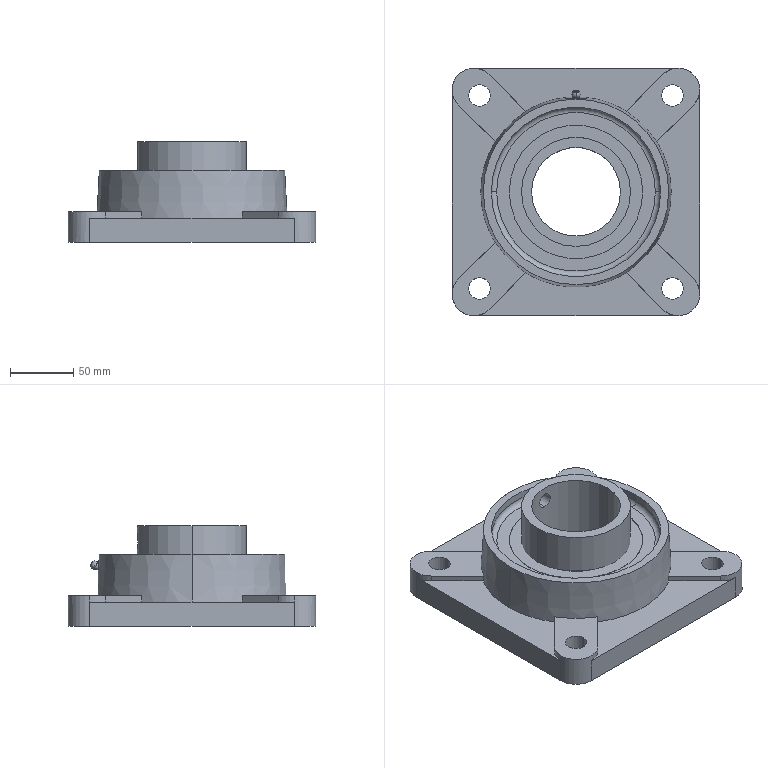Part | SolidWorks | features Revolution 5, Boss 2, RevCut 2, CirPattern 1, Cut 1, Extrusion 1, RefAxis 1 | 18 solids | 148 faces | box 195 x 195 x 79.4 mm | volume 823685 mm3 | cylinder 58 | plane 38 | sphere 38 | torus 12 | cone 2 | commonest cylinder face diameters 34 x12 6 x10 17 x8 105.2 x8 84.95 x4 85.95 x4